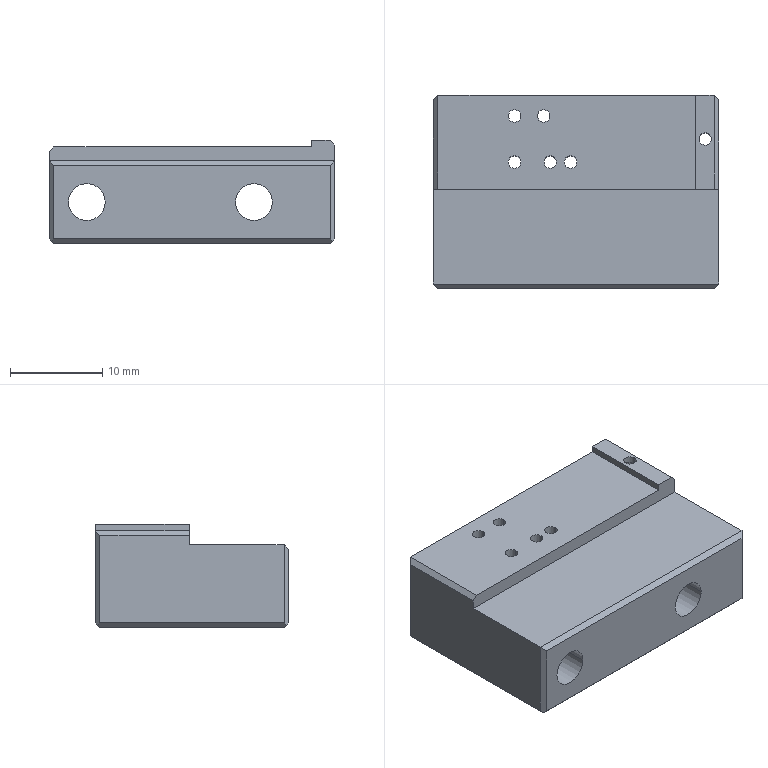Part | 1 solid | 45 faces | box 31 x 21 x 11.2 mm | volume 5581 mm3 | plane 23 | cylinder 22 | commonest cylinder face diameters 1.35 x14 4 x4 6 x2 6.5 x2
STEP:
#1=CARTESIAN_POINT('',(2008.3,163.,-157.1));
#2=VERTEX_POINT('',#1);
#3=CARTESIAN_POINT('',(2008.3,163.,-167.3));
#4=VERTEX_POINT('',#3);
#5=CARTESIAN_POINT('',(2008.3,163.,-162.2));
#6=DIRECTION('',(0.,0.,-1.));
#7=VECTOR('',#6,1000.);
#8=LINE('',#5,#7);
#9=EDGE_CURVE('',#2,#4,#8,.T.);
#10=ORIENTED_EDGE('',*,*,#9,.F.);
#11=CARTESIAN_POINT('',(2008.3,153.3,-157.1));
#12=VERTEX_POINT('',#11);
#13=CARTESIAN_POINT('',(2008.3,158.4,-157.1));
#14=DIRECTION('',(0.,1.,0.));
#15=VECTOR('',#14,1000.);
#16=LINE('',#13,#15);
#17=EDGE_CURVE('',#12,#2,#16,.T.);
#18=ORIENTED_EDGE('',*,*,#17,.F.);
#19=CARTESIAN_POINT('',(2008.3,153.3,-158.8));
#20=VERTEX_POINT('',#19);
#21=CARTESIAN_POINT('',(2008.3,153.3,-197.47));
#22=DIRECTION('',(0.,0.,-1.));
#23=VECTOR('',#22,1000.);
#24=LINE('',#21,#23);
#25=EDGE_CURVE('',#12,#20,#24,.T.);
#26=ORIENTED_EDGE('',*,*,#25,.T.);
#27=CARTESIAN_POINT('',(2008.3,143.,-158.8));
#28=VERTEX_POINT('',#27);
#29=CARTESIAN_POINT('',(2008.3,142.5,-158.8));
#30=DIRECTION('',(0.,-1.,0.));
#31=VECTOR('',#30,1000.);
#32=LINE('',#29,#31);
#33=EDGE_CURVE('',#20,#28,#32,.T.);
#34=ORIENTED_EDGE('',*,*,#33,.T.);
#35=CARTESIAN_POINT('',(2008.3,143.,-167.3));
#36=VERTEX_POINT('',#35);
#37=CARTESIAN_POINT('',(2008.3,143.,-163.05));
#38=DIRECTION('',(0.,0.,-1.));
#39=VECTOR('',#38,1000.);
#40=LINE('',#37,#39);
#41=EDGE_CURVE('',#28,#36,#40,.T.);
#42=ORIENTED_EDGE('',*,*,#41,.T.);
#43=CARTESIAN_POINT('',(2008.3,153.,-167.3));
#44=DIRECTION('',(0.,-1.,0.));
#45=VECTOR('',#44,1000.);
#46=LINE('',#43,#45);
#47=EDGE_CURVE('',#4,#36,#46,.T.);
#48=ORIENTED_EDGE('',*,*,#47,.F.);
#49=EDGE_LOOP('',(#10,#18,#26,#34,#42,#48));
#50=FACE_BOUND('',#49,.T.);
#51=CARTESIAN_POINT('',(2008.3,142.5,-213.5));
#52=DIRECTION('',(1.,0.,0.));
#53=DIRECTION('',(0.,1.,0.));
#54=AXIS2_PLACEMENT_3D('',#51,#52,#53);
#55=PLANE('',#54);
#56=ADVANCED_FACE('',(#50),#55,.T.);
#57=CARTESIAN_POINT('',(1977.8,143.,-167.8));
#58=VERTEX_POINT('',#57);
#59=CARTESIAN_POINT('',(1977.8,163.,-167.8));
#60=VERTEX_POINT('',#59);
#61=CARTESIAN_POINT('',(1977.8,153.,-167.8));
#62=DIRECTION('',(0.,1.,0.));
#63=VECTOR('',#62,1000.);
#64=LINE('',#61,#63);
#65=EDGE_CURVE('',#58,#60,#64,.T.);
#66=ORIENTED_EDGE('',*,*,#65,.T.);
#67=CARTESIAN_POINT('',(2007.8,163.,-167.8));
#68=VERTEX_POINT('',#67);
#69=CARTESIAN_POINT('',(1992.8,163.,-167.8));
#70=DIRECTION('',(1.,0.,0.));
#71=VECTOR('',#70,1000.);
#72=LINE('',#69,#71);
#73=EDGE_CURVE('',#60,#68,#72,.T.);
#74=ORIENTED_EDGE('',*,*,#73,.T.);
#75=CARTESIAN_POINT('',(2007.8,143.,-167.8));
#76=VERTEX_POINT('',#75);
#77=CARTESIAN_POINT('',(2007.8,153.,-167.8));
#78=DIRECTION('',(0.,-1.,0.));
#79=VECTOR('',#78,1000.);
#80=LINE('',#77,#79);
#81=EDGE_CURVE('',#68,#76,#80,.T.);
#82=ORIENTED_EDGE('',*,*,#81,.T.);
#83=CARTESIAN_POINT('',(1992.8,143.,-167.8));
#84=DIRECTION('',(-1.,0.,0.));
#85=VECTOR('',#84,1000.);
#86=LINE('',#83,#85);
#87=EDGE_CURVE('',#76,#58,#86,.T.);
#88=ORIENTED_EDGE('',*,*,#87,.T.);
#89=EDGE_LOOP('',(#66,#74,#82,#88));
#90=FACE_BOUND('',#89,.T.);
#91=CARTESIAN_POINT('',(1986.795,156.238,-167.8));
#92=VERTEX_POINT('',#91);
#93=CARTESIAN_POINT('',(1985.445,156.238,-167.8));
#94=VERTEX_POINT('',#93);
#95=CARTESIAN_POINT('',(1986.12,156.238,-167.8));
#96=DIRECTION('',(0.,0.,1.));
#97=DIRECTION('',(-1.,0.,0.));
#98=AXIS2_PLACEMENT_3D('',#95,#96,#97);
#99=CIRCLE('',#98,0.675);
#100=EDGE_CURVE('',#92,#94,#99,.T.);
#101=ORIENTED_EDGE('',*,*,#100,.T.);
#102=CARTESIAN_POINT('',(1986.12,156.238,-167.8));
#103=DIRECTION('',(0.,0.,1.));
#104=DIRECTION('',(-1.,0.,0.));
#105=AXIS2_PLACEMENT_3D('',#102,#103,#104);
#106=CIRCLE('',#105,0.675);
#107=EDGE_CURVE('',#94,#92,#106,.T.);
#108=ORIENTED_EDGE('',*,*,#107,.T.);
#109=EDGE_LOOP('',(#101,#108));
#110=FACE_BOUND('',#109,.T.);
#111=CARTESIAN_POINT('',(1992.885,156.238,-167.8));
#112=VERTEX_POINT('',#111);
#113=CARTESIAN_POINT('',(1991.535,156.238,-167.8));
#114=VERTEX_POINT('',#113);
#115=CARTESIAN_POINT('',(1992.21,156.238,-167.8));
#116=DIRECTION('',(0.,0.,1.));
#117=DIRECTION('',(-1.,0.,0.));
#118=AXIS2_PLACEMENT_3D('',#115,#116,#117);
#119=CIRCLE('',#118,0.675);
#120=EDGE_CURVE('',#112,#114,#119,.T.);
#121=ORIENTED_EDGE('',*,*,#120,.T.);
#122=CARTESIAN_POINT('',(1992.21,156.238,-167.8));
#123=DIRECTION('',(0.,0.,1.));
#124=DIRECTION('',(-1.,0.,0.));
#125=AXIS2_PLACEMENT_3D('',#122,#123,#124);
#126=CIRCLE('',#125,0.675);
#127=EDGE_CURVE('',#114,#112,#126,.T.);
#128=ORIENTED_EDGE('',*,*,#127,.T.);
#129=EDGE_LOOP('',(#121,#128));
#130=FACE_BOUND('',#129,.T.);
#131=CARTESIAN_POINT('',(2007.525,158.748,-167.8));
#132=VERTEX_POINT('',#131);
#133=CARTESIAN_POINT('',(2006.175,158.748,-167.8));
#134=VERTEX_POINT('',#133);
#135=CARTESIAN_POINT('',(2006.85,158.748,-167.8));
#136=DIRECTION('',(0.,0.,-1.));
#137=DIRECTION('',(-1.,0.,0.));
#138=AXIS2_PLACEMENT_3D('',#135,#136,#137);
#139=CIRCLE('',#138,0.675);
#140=EDGE_CURVE('',#132,#134,#139,.T.);
#141=ORIENTED_EDGE('',*,*,#140,.F.);
#142=CARTESIAN_POINT('',(2006.85,158.748,-167.8));
#143=DIRECTION('',(0.,0.,-1.));
#144=DIRECTION('',(-1.,0.,0.));
#145=AXIS2_PLACEMENT_3D('',#142,#143,#144);
#146=CIRCLE('',#145,0.675);
#147=EDGE_CURVE('',#134,#132,#146,.T.);
#148=ORIENTED_EDGE('',*,*,#147,.F.);
#149=EDGE_LOOP('',(#141,#148));
#150=FACE_BOUND('',#149,.T.);
#151=CARTESIAN_POINT('',(1986.795,161.259,-167.8));
#152=VERTEX_POINT('',#151);
#153=CARTESIAN_POINT('',(1985.445,161.259,-167.8));
#154=VERTEX_POINT('',#153);
#155=CARTESIAN_POINT('',(1986.12,161.259,-167.8));
#156=DIRECTION('',(0.,0.,1.));
#157=DIRECTION('',(-1.,0.,0.));
#158=AXIS2_PLACEMENT_3D('',#155,#156,#157);
#159=CIRCLE('',#158,0.675);
#160=EDGE_CURVE('',#152,#154,#159,.T.);
#161=ORIENTED_EDGE('',*,*,#160,.T.);
#162=CARTESIAN_POINT('',(1986.12,161.259,-167.8));
#163=DIRECTION('',(0.,0.,1.));
#164=DIRECTION('',(-1.,0.,0.));
#165=AXIS2_PLACEMENT_3D('',#162,#163,#164);
#166=CIRCLE('',#165,0.675);
#167=EDGE_CURVE('',#154,#152,#166,.T.);
#168=ORIENTED_EDGE('',*,*,#167,.T.);
#169=EDGE_LOOP('',(#161,#168));
#170=FACE_BOUND('',#169,.T.);
#171=CARTESIAN_POINT('',(1989.958,161.259,-167.8));
#172=VERTEX_POINT('',#171);
#173=CARTESIAN_POINT('',(1988.608,161.259,-167.8));
#174=VERTEX_POINT('',#173);
#175=CARTESIAN_POINT('',(1989.283,161.259,-167.8));
#176=DIRECTION('',(0.,0.,1.));
#177=DIRECTION('',(-1.,0.,0.));
#178=AXIS2_PLACEMENT_3D('',#175,#176,#177);
#179=CIRCLE('',#178,0.675);
#180=EDGE_CURVE('',#172,#174,#179,.T.);
#181=ORIENTED_EDGE('',*,*,#180,.T.);
#182=CARTESIAN_POINT('',(1989.283,161.259,-167.8));
#183=DIRECTION('',(0.,0.,1.));
#184=DIRECTION('',(-1.,0.,0.));
#185=AXIS2_PLACEMENT_3D('',#182,#183,#184);
#186=CIRCLE('',#185,0.675);
#187=EDGE_CURVE('',#174,#172,#186,.T.);
#188=ORIENTED_EDGE('',*,*,#187,.T.);
#189=EDGE_LOOP('',(#181,#188));
#190=FACE_BOUND('',#189,.T.);
#191=CARTESIAN_POINT('',(1990.685,156.238,-167.8));
#192=VERTEX_POINT('',#191);
#193=CARTESIAN_POINT('',(1989.335,156.238,-167.8));
#194=VERTEX_POINT('',#193);
#195=CARTESIAN_POINT('',(1990.01,156.238,-167.8));
#196=DIRECTION('',(0.,0.,1.));
#197=DIRECTION('',(-1.,0.,0.));
#198=AXIS2_PLACEMENT_3D('',#195,#196,#197);
#199=CIRCLE('',#198,0.675);
#200=EDGE_CURVE('',#192,#194,#199,.T.);
#201=ORIENTED_EDGE('',*,*,#200,.T.);
#202=CARTESIAN_POINT('',(1990.01,156.238,-167.8));
#203=DIRECTION('',(0.,0.,1.));
#204=DIRECTION('',(-1.,0.,0.));
#205=AXIS2_PLACEMENT_3D('',#202,#203,#204);
#206=CIRCLE('',#205,0.675);
#207=EDGE_CURVE('',#194,#192,#206,.T.);
#208=ORIENTED_EDGE('',*,*,#207,.T.);
#209=EDGE_LOOP('',(#201,#208));
#210=FACE_BOUND('',#209,.T.);
#211=CARTESIAN_POINT('',(2010.,142.5,-167.8));
#212=DIRECTION('',(0.,0.,-1.));
#213=DIRECTION('',(0.,-1.,0.));
#214=AXIS2_PLACEMENT_3D('',#211,#212,#213);
#215=PLANE('',#214);
#216=ADVANCED_FACE('',(#90,#110,#130,#150,#170,#190,#210),#215,.T.);
#217=CARTESIAN_POINT('',(1977.3,163.,-157.8));
#218=VERTEX_POINT('',#217);
#219=CARTESIAN_POINT('',(1977.3,153.3,-157.8));
#220=VERTEX_POINT('',#219);
#221=CARTESIAN_POINT('',(1977.3,158.4,-157.8));
#222=DIRECTION('',(0.,-1.,0.));
#223=VECTOR('',#222,1000.);
#224=LINE('',#221,#223);
#225=EDGE_CURVE('',#218,#220,#224,.T.);
#226=ORIENTED_EDGE('',*,*,#225,.F.);
#227=CARTESIAN_POINT('',(1977.3,163.,-167.3));
#228=VERTEX_POINT('',#227);
#229=CARTESIAN_POINT('',(1977.3,163.,-162.55));
#230=DIRECTION('',(0.,0.,1.));
#231=VECTOR('',#230,1000.);
#232=LINE('',#229,#231);
#233=EDGE_CURVE('',#228,#218,#232,.T.);
#234=ORIENTED_EDGE('',*,*,#233,.F.);
#235=CARTESIAN_POINT('',(1977.3,143.,-167.3));
#236=VERTEX_POINT('',#235);
#237=CARTESIAN_POINT('',(1977.3,153.,-167.3));
#238=DIRECTION('',(0.,1.,0.));
#239=VECTOR('',#238,1000.);
#240=LINE('',#237,#239);
#241=EDGE_CURVE('',#236,#228,#240,.T.);
#242=ORIENTED_EDGE('',*,*,#241,.F.);
#243=CARTESIAN_POINT('',(1977.3,143.,-158.8));
#244=VERTEX_POINT('',#243);
#245=CARTESIAN_POINT('',(1977.3,143.,-163.05));
#246=DIRECTION('',(0.,0.,1.));
#247=VECTOR('',#246,1000.);
#248=LINE('',#245,#247);
#249=EDGE_CURVE('',#236,#244,#248,.T.);
#250=ORIENTED_EDGE('',*,*,#249,.T.);
#251=CARTESIAN_POINT('',(1977.3,153.3,-158.8));
#252=VERTEX_POINT('',#251);
#253=CARTESIAN_POINT('',(1977.3,142.5,-158.8));
#254=DIRECTION('',(0.,1.,0.));
#255=VECTOR('',#254,1000.);
#256=LINE('',#253,#255);
#257=EDGE_CURVE('',#244,#252,#256,.T.);
#258=ORIENTED_EDGE('',*,*,#257,.T.);
#259=CARTESIAN_POINT('',(1977.3,153.3,-197.47));
#260=DIRECTION('',(0.,0.,1.));
#261=VECTOR('',#260,1000.);
#262=LINE('',#259,#261);
#263=EDGE_CURVE('',#252,#220,#262,.T.);
#264=ORIENTED_EDGE('',*,*,#263,.T.);
#265=EDGE_LOOP('',(#226,#234,#242,#250,#258,#264));
#266=FACE_BOUND('',#265,.T.);
#267=CARTESIAN_POINT('',(1977.3,142.5,-205.7));
#268=DIRECTION('',(-1.,0.,0.));
#269=DIRECTION('',(0.,0.,1.));
#270=AXIS2_PLACEMENT_3D('',#267,#268,#269);
#271=PLANE('',#270);
#272=ADVANCED_FACE('',(#266),#271,.T.);
#273=CARTESIAN_POINT('',(2005.8,153.3,-156.6));
#274=VERTEX_POINT('',#273);
#275=CARTESIAN_POINT('',(2005.8,153.3,-157.3));
#276=VERTEX_POINT('',#275);
#277=CARTESIAN_POINT('',(2005.8,153.3,-197.47));
#278=DIRECTION('',(0.,0.,-1.));
#279=VECTOR('',#278,1000.);
#280=LINE('',#277,#279);
#281=EDGE_CURVE('',#274,#276,#280,.T.);
#282=ORIENTED_EDGE('',*,*,#281,.F.);
#283=CARTESIAN_POINT('',(2005.8,163.5,-156.6));
#284=VERTEX_POINT('',#283);
#285=CARTESIAN_POINT('',(2005.8,142.5,-156.6));
#286=DIRECTION('',(0.,1.,0.));
#287=VECTOR('',#286,1000.);
#288=LINE('',#285,#287);
#289=EDGE_CURVE('',#274,#284,#288,.T.);
#290=ORIENTED_EDGE('',*,*,#289,.T.);
#291=CARTESIAN_POINT('',(2005.8,163.5,-157.3));
#292=VERTEX_POINT('',#291);
#293=CARTESIAN_POINT('',(2005.8,163.5,-197.47));
#294=DIRECTION('',(0.,0.,-1.));
#295=VECTOR('',#294,1000.);
#296=LINE('',#293,#295);
#297=EDGE_CURVE('',#284,#292,#296,.T.);
#298=ORIENTED_EDGE('',*,*,#297,.T.);
#299=CARTESIAN_POINT('',(2005.8,142.5,-157.3));
#300=DIRECTION('',(0.,-1.,0.));
#301=VECTOR('',#300,1000.);
#302=LINE('',#299,#301);
#303=EDGE_CURVE('',#292,#276,#302,.T.);
#304=ORIENTED_EDGE('',*,*,#303,.T.);
#305=EDGE_LOOP('',(#282,#290,#298,#304));
#306=FACE_BOUND('',#305,.T.);
#307=CARTESIAN_POINT('',(2005.8,142.5,-157.3));
#308=DIRECTION('',(-1.,0.,0.));
#309=DIRECTION('',(0.,0.,1.));
#310=AXIS2_PLACEMENT_3D('',#307,#308,#309);
#311=PLANE('',#310);
#312=ADVANCED_FACE('',(#306),#311,.T.);
#313=CARTESIAN_POINT('',(1986.795,161.259,-157.3));
#314=VERTEX_POINT('',#313);
#315=CARTESIAN_POINT('',(1985.445,161.259,-157.3));
#316=VERTEX_POINT('',#315);
#317=CARTESIAN_POINT('',(1986.12,161.259,-157.3));
#318=DIRECTION('',(0.,0.,1.));
#319=DIRECTION('',(-1.,0.,0.));
#320=AXIS2_PLACEMENT_3D('',#317,#318,#319);
#321=CIRCLE('',#320,0.675);
#322=EDGE_CURVE('',#314,#316,#321,.T.);
#323=ORIENTED_EDGE('',*,*,#322,.T.);
#324=CARTESIAN_POINT('',(1985.445,161.259,-157.3));
#325=DIRECTION('',(0.,0.,1.));
#326=VECTOR('',#325,1000.);
#327=LINE('',#324,#326);
#328=EDGE_CURVE('',#316,#154,#327,.F.);
#329=ORIENTED_EDGE('',*,*,#328,.T.);
#330=ORIENTED_EDGE('',*,*,#160,.F.);
#331=CARTESIAN_POINT('',(1986.795,161.259,-157.3));
#332=DIRECTION('',(0.,0.,1.));
#333=VECTOR('',#332,1000.);
#334=LINE('',#331,#333);
#335=EDGE_CURVE('',#314,#152,#334,.F.);
#336=ORIENTED_EDGE('',*,*,#335,.F.);
#337=EDGE_LOOP('',(#323,#329,#330,#336));
#338=FACE_BOUND('',#337,.T.);
#339=CARTESIAN_POINT('',(1986.12,161.259,-157.3));
#340=DIRECTION('',(0.,0.,1.));
#341=DIRECTION('',(-1.,0.,0.));
#342=AXIS2_PLACEMENT_3D('',#339,#340,#341);
#343=CYLINDRICAL_SURFACE('',#342,0.675);
#344=ADVANCED_FACE('',(#338),#343,.F.);
#345=CARTESIAN_POINT('',(1989.958,161.259,-157.3));
#346=VERTEX_POINT('',#345);
#347=CARTESIAN_POINT('',(1988.608,161.259,-157.3));
#348=VERTEX_POINT('',#347);
#349=CARTESIAN_POINT('',(1989.283,161.259,-157.3));
#350=DIRECTION('',(0.,0.,1.));
#351=DIRECTION('',(-1.,0.,0.));
#352=AXIS2_PLACEMENT_3D('',#349,#350,#351);
#353=CIRCLE('',#352,0.675);
#354=EDGE_CURVE('',#346,#348,#353,.T.);
#355=ORIENTED_EDGE('',*,*,#354,.T.);
#356=CARTESIAN_POINT('',(1988.608,161.259,-157.3));
#357=DIRECTION('',(0.,0.,1.));
#358=VECTOR('',#357,1000.);
#359=LINE('',#356,#358);
#360=EDGE_CURVE('',#348,#174,#359,.F.);
#361=ORIENTED_EDGE('',*,*,#360,.T.);
#362=ORIENTED_EDGE('',*,*,#180,.F.);
#363=CARTESIAN_POINT('',(1989.958,161.259,-157.3));
#364=DIRECTION('',(0.,0.,1.));
#365=VECTOR('',#364,1000.);
#366=LINE('',#363,#365);
#367=EDGE_CURVE('',#346,#172,#366,.F.);
#368=ORIENTED_EDGE('',*,*,#367,.F.);
#369=EDGE_LOOP('',(#355,#361,#362,#368));
#370=FACE_BOUND('',#369,.T.);
#371=CARTESIAN_POINT('',(1989.283,161.259,-157.3));
#372=DIRECTION('',(0.,0.,1.));
#373=DIRECTION('',(-1.,0.,0.));
#374=AXIS2_PLACEMENT_3D('',#371,#372,#373);
#375=CYLINDRICAL_SURFACE('',#374,0.675);
#376=ADVANCED_FACE('',(#370),#375,.F.);
#377=CARTESIAN_POINT('',(1990.685,156.238,-157.3));
#378=VERTEX_POINT('',#377);
#379=CARTESIAN_POINT('',(1989.335,156.238,-157.3));
#380=VERTEX_POINT('',#379);
#381=CARTESIAN_POINT('',(1990.01,156.238,-157.3));
#382=DIRECTION('',(0.,0.,1.));
#383=DIRECTION('',(-1.,0.,0.));
#384=AXIS2_PLACEMENT_3D('',#381,#382,#383);
#385=CIRCLE('',#384,0.675);
#386=EDGE_CURVE('',#378,#380,#385,.T.);
#387=ORIENTED_EDGE('',*,*,#386,.T.);
#388=CARTESIAN_POINT('',(1989.335,156.238,-157.3));
#389=DIRECTION('',(0.,0.,1.));
#390=VECTOR('',#389,1000.);
#391=LINE('',#388,#390);
#392=EDGE_CURVE('',#380,#194,#391,.F.);
#393=ORIENTED_EDGE('',*,*,#392,.T.);
#394=ORIENTED_EDGE('',*,*,#200,.F.);
#395=CARTESIAN_POINT('',(1990.685,156.238,-157.3));
#396=DIRECTION('',(0.,0.,1.));
#397=VECTOR('',#396,1000.);
#398=LINE('',#395,#397);
#399=EDGE_CURVE('',#378,#192,#398,.F.);
#400=ORIENTED_EDGE('',*,*,#399,.F.);
#401=EDGE_LOOP('',(#387,#393,#394,#400));
#402=FACE_BOUND('',#401,.T.);
#403=CARTESIAN_POINT('',(1990.01,156.238,-157.3));
#404=DIRECTION('',(0.,0.,1.));
#405=DIRECTION('',(-1.,0.,0.));
#406=AXIS2_PLACEMENT_3D('',#403,#404,#405);
#407=CYLINDRICAL_SURFACE('',#406,0.675);
#408=ADVANCED_FACE('',(#402),#407,.F.);
#409=CARTESIAN_POINT('',(1986.795,156.238,-157.3));
#410=VERTEX_POINT('',#409);
#411=CARTESIAN_POINT('',(1985.445,156.238,-157.3));
#412=VERTEX_POINT('',#411);
#413=CARTESIAN_POINT('',(1986.12,156.238,-157.3));
#414=DIRECTION('',(0.,0.,1.));
#415=DIRECTION('',(-1.,0.,0.));
#416=AXIS2_PLACEMENT_3D('',#413,#414,#415);
#417=CIRCLE('',#416,0.675);
#418=EDGE_CURVE('',#410,#412,#417,.T.);
#419=ORIENTED_EDGE('',*,*,#418,.T.);
#420=CARTESIAN_POINT('',(1985.445,156.238,-157.3));
#421=DIRECTION('',(0.,0.,1.));
#422=VECTOR('',#421,1000.);
#423=LINE('',#420,#422);
#424=EDGE_CURVE('',#412,#94,#423,.F.);
#425=ORIENTED_EDGE('',*,*,#424,.T.);
#426=ORIENTED_EDGE('',*,*,#100,.F.);
#427=CARTESIAN_POINT('',(1986.795,156.238,-157.3));
#428=DIRECTION('',(0.,0.,1.));
#429=VECTOR('',#428,1000.);
#430=LINE('',#427,#429);
#431=EDGE_CURVE('',#410,#92,#430,.F.);
#432=ORIENTED_EDGE('',*,*,#431,.F.);
#433=EDGE_LOOP('',(#419,#425,#426,#432));
#434=FACE_BOUND('',#433,.T.);
#435=CARTESIAN_POINT('',(1986.12,156.238,-157.3));
#436=DIRECTION('',(0.,0.,1.));
#437=DIRECTION('',(-1.,0.,0.));
#438=AXIS2_PLACEMENT_3D('',#435,#436,#437);
#439=CYLINDRICAL_SURFACE('',#438,0.675);
#440=ADVANCED_FACE('',(#434),#439,.F.);
#441=CARTESIAN_POINT('',(1992.885,156.238,-157.3));
#442=VERTEX_POINT('',#441);
#443=CARTESIAN_POINT('',(1991.535,156.238,-157.3));
#444=VERTEX_POINT('',#443);
#445=CARTESIAN_POINT('',(1992.21,156.238,-157.3));
#446=DIRECTION('',(0.,0.,1.));
#447=DIRECTION('',(-1.,0.,0.));
#448=AXIS2_PLACEMENT_3D('',#445,#446,#447);
#449=CIRCLE('',#448,0.675);
#450=EDGE_CURVE('',#442,#444,#449,.T.);
#451=ORIENTED_EDGE('',*,*,#450,.T.);
#452=CARTESIAN_POINT('',(1991.535,156.238,-157.3));
#453=DIRECTION('',(0.,0.,1.));
#454=VECTOR('',#453,1000.);
#455=LINE('',#452,#454);
#456=EDGE_CURVE('',#444,#114,#455,.F.);
#457=ORIENTED_EDGE('',*,*,#456,.T.);
#458=ORIENTED_EDGE('',*,*,#120,.F.);
#459=CARTESIAN_POINT('',(1992.885,156.238,-157.3));
#460=DIRECTION('',(0.,0.,1.));
#461=VECTOR('',#460,1000.);
#462=LINE('',#459,#461);
#463=EDGE_CURVE('',#442,#112,#462,.F.);
#464=ORIENTED_EDGE('',*,*,#463,.F.);
#465=EDGE_LOOP('',(#451,#457,#458,#464));
#466=FACE_BOUND('',#465,.T.);
#467=CARTESIAN_POINT('',(1992.21,156.238,-157.3));
#468=DIRECTION('',(0.,0.,1.));
#469=DIRECTION('',(-1.,0.,0.));
#470=AXIS2_PLACEMENT_3D('',#467,#468,#469);
#471=CYLINDRICAL_SURFACE('',#470,0.675);
#472=ADVANCED_FACE('',(#466),#471,.F.);
#473=CARTESIAN_POINT('',(2007.525,158.748,-157.3));
#474=VERTEX_POINT('',#473);
#475=CARTESIAN_POINT('',(2006.175,158.748,-157.3));
#476=VERTEX_POINT('',#475);
#477=CARTESIAN_POINT('',(2006.85,158.748,-157.3));
#478=DIRECTION('',(0.,0.,-1.));
#479=DIRECTION('',(-1.,0.,0.));
#480=AXIS2_PLACEMENT_3D('',#477,#478,#479);
#481=CIRCLE('',#480,0.675);
#482=EDGE_CURVE('',#474,#476,#481,.T.);
#483=ORIENTED_EDGE('',*,*,#482,.F.);
#484=CARTESIAN_POINT('',(2007.525,158.748,-157.3));
#485=DIRECTION('',(0.,0.,1.));
#486=VECTOR('',#485,1000.);
#487=LINE('',#484,#486);
#488=EDGE_CURVE('',#474,#132,#487,.F.);
#489=ORIENTED_EDGE('',*,*,#488,.T.);
#490=ORIENTED_EDGE('',*,*,#140,.T.);
#491=CARTESIAN_POINT('',(2006.175,158.748,-157.3));
#492=DIRECTION('',(0.,0.,1.));
#493=VECTOR('',#492,1000.);
#494=LINE('',#491,#493);
#495=EDGE_CURVE('',#476,#134,#494,.F.);
#496=ORIENTED_EDGE('',*,*,#495,.F.);
#497=EDGE_LOOP('',(#483,#489,#490,#496));
#498=FACE_BOUND('',#497,.T.);
#499=CARTESIAN_POINT('',(2006.85,158.748,-157.3));
#500=DIRECTION('',(0.,0.,1.));
#501=DIRECTION('',(-1.,0.,0.));
#502=AXIS2_PLACEMENT_3D('',#499,#500,#501);
#503=CYLINDRICAL_SURFACE('',#502,0.675);
#504=ADVANCED_FACE('',(#498),#503,.F.);
#505=CARTESIAN_POINT('',(1977.8,153.3,-157.3));
#506=VERTEX_POINT('',#505);
#507=CARTESIAN_POINT('',(1983.678,153.3,-157.3));
#508=DIRECTION('',(-1.,0.,0.));
#509=VECTOR('',#508,1000.);
#510=LINE('',#507,#509);
#511=EDGE_CURVE('',#276,#506,#510,.T.);
#512=ORIENTED_EDGE('',*,*,#511,.F.);
#513=ORIENTED_EDGE('',*,*,#303,.F.);
#514=CARTESIAN_POINT('',(1977.8,163.5,-157.3));
#515=VERTEX_POINT('',#514);
#516=CARTESIAN_POINT('',(1983.678,163.5,-157.3));
#517=DIRECTION('',(-1.,0.,0.));
#518=VECTOR('',#517,1000.);
#519=LINE('',#516,#518);
#520=EDGE_CURVE('',#292,#515,#519,.T.);
#521=ORIENTED_EDGE('',*,*,#520,.T.);
#522=CARTESIAN_POINT('',(1977.8,158.4,-157.3));
#523=DIRECTION('',(0.,-1.,0.));
#524=VECTOR('',#523,1000.);
#525=LINE('',#522,#524);
#526=EDGE_CURVE('',#515,#506,#525,.T.);
#527=ORIENTED_EDGE('',*,*,#526,.T.);
#528=EDGE_LOOP('',(#512,#513,#521,#527));
#529=FACE_BOUND('',#528,.T.);
#530=ORIENTED_EDGE('',*,*,#450,.F.);
#531=CARTESIAN_POINT('',(1992.21,156.238,-157.3));
#532=DIRECTION('',(0.,0.,1.));
#533=DIRECTION('',(-1.,0.,0.));
#534=AXIS2_PLACEMENT_3D('',#531,#532,#533);
#535=CIRCLE('',#534,0.675);
#536=EDGE_CURVE('',#444,#442,#535,.T.);
#537=ORIENTED_EDGE('',*,*,#536,.F.);
#538=EDGE_LOOP('',(#530,#537));
#539=FACE_BOUND('',#538,.T.);
#540=ORIENTED_EDGE('',*,*,#322,.F.);
#541=CARTESIAN_POINT('',(1986.12,161.259,-157.3));
#542=DIRECTION('',(0.,0.,1.));
#543=DIRECTION('',(-1.,0.,0.));
#544=AXIS2_PLACEMENT_3D('',#541,#542,#543);
#545=CIRCLE('',#544,0.675);
#546=EDGE_CURVE('',#316,#314,#545,.T.);
#547=ORIENTED_EDGE('',*,*,#546,.F.);
#548=EDGE_LOOP('',(#540,#547));
#549=FACE_BOUND('',#548,.T.);
#550=ORIENTED_EDGE('',*,*,#354,.F.);
#551=CARTESIAN_POINT('',(1989.283,161.259,-157.3));
#552=DIRECTION('',(0.,0.,1.));
#553=DIRECTION('',(-1.,0.,0.));
#554=AXIS2_PLACEMENT_3D('',#551,#552,#553);
#555=CIRCLE('',#554,0.675);
#556=EDGE_CURVE('',#348,#346,#555,.T.);
#557=ORIENTED_EDGE('',*,*,#556,.F.);
#558=EDGE_LOOP('',(#550,#557));
#559=FACE_BOUND('',#558,.T.);
#560=ORIENTED_EDGE('',*,*,#386,.F.);
#561=CARTESIAN_POINT('',(1990.01,156.238,-157.3));
#562=DIRECTION('',(0.,0.,1.));
#563=DIRECTION('',(-1.,0.,0.));
#564=AXIS2_PLACEMENT_3D('',#561,#562,#563);
#565=CIRCLE('',#564,0.675);
#566=EDGE_CURVE('',#380,#378,#565,.T.);
#567=ORIENTED_EDGE('',*,*,#566,.F.);
#568=EDGE_LOOP('',(#560,#567));
#569=FACE_BOUND('',#568,.T.);
#570=ORIENTED_EDGE('',*,*,#418,.F.);
#571=CARTESIAN_POINT('',(1986.12,156.238,-157.3));
#572=DIRECTION('',(0.,0.,1.));
#573=DIRECTION('',(-1.,0.,0.));
#574=AXIS2_PLACEMENT_3D('',#571,#572,#573);
#575=CIRCLE('',#574,0.675);
#576=EDGE_CURVE('',#412,#410,#575,.T.);
#577=ORIENTED_EDGE('',*,*,#576,.F.);
#578=EDGE_LOOP('',(#570,#577));
#579=FACE_BOUND('',#578,.T.);
#580=CARTESIAN_POINT('',(2010.3,142.5,-157.3));
#581=DIRECTION('',(0.,0.,1.));
#582=DIRECTION('',(1.,0.,0.));
#583=AXIS2_PLACEMENT_3D('',#580,#581,#582);
#584=PLANE('',#583);
#585=ADVANCED_FACE('',(#529,#539,#549,#559,#569,#579),#584,.T.);
#586=CARTESIAN_POINT('',(2007.8,153.3,-156.6));
#587=VERTEX_POINT('',#586);
#588=CARTESIAN_POINT('',(2007.8,163.5,-156.6));
#589=VERTEX_POINT('',#588);
#590=CARTESIAN_POINT('',(2007.8,158.4,-156.6));
#591=DIRECTION('',(0.,1.,0.));
#592=VECTOR('',#591,1000.);
#593=LINE('',#590,#592);
#594=EDGE_CURVE('',#587,#589,#593,.T.);
#595=ORIENTED_EDGE('',*,*,#594,.T.);
#596=CARTESIAN_POINT('',(1983.678,163.5,-156.6));
#597=DIRECTION('',(-1.,0.,0.));
#598=VECTOR('',#597,1000.);
#599=LINE('',#596,#598);
#600=EDGE_CURVE('',#589,#284,#599,.T.);
#601=ORIENTED_EDGE('',*,*,#600,.T.);
#602=ORIENTED_EDGE('',*,*,#289,.F.);
#603=CARTESIAN_POINT('',(1983.678,153.3,-156.6));
#604=DIRECTION('',(-1.,0.,0.));
#605=VECTOR('',#604,1000.);
#606=LINE('',#603,#605);
#607=EDGE_CURVE('',#587,#274,#606,.T.);
#608=ORIENTED_EDGE('',*,*,#607,.F.);
#609=EDGE_LOOP('',(#595,#601,#602,#608));
#610=FACE_BOUND('',#609,.T.);
#611=CARTESIAN_POINT('',(2007.525,158.748,-156.6));
#612=VERTEX_POINT('',#611);
#613=CARTESIAN_POINT('',(2006.175,158.748,-156.6));
#614=VERTEX_POINT('',#613);
#615=CARTESIAN_POINT('',(2006.85,158.748,-156.6));
#616=DIRECTION('',(0.,0.,-1.));
#617=DIRECTION('',(-1.,0.,0.));
#618=AXIS2_PLACEMENT_3D('',#615,#616,#617);
#619=CIRCLE('',#618,0.675);
#620=EDGE_CURVE('',#612,#614,#619,.T.);
#621=ORIENTED_EDGE('',*,*,#620,.T.);
#622=CARTESIAN_POINT('',(2006.85,158.748,-156.6));
#623=DIRECTION('',(0.,0.,-1.));
#624=DIRECTION('',(-1.,0.,0.));
#625=AXIS2_PLACEMENT_3D('',#622,#623,#624);
#626=CIRCLE('',#625,0.675);
#627=EDGE_CURVE('',#614,#612,#626,.T.);
#628=ORIENTED_EDGE('',*,*,#627,.T.);
#629=EDGE_LOOP('',(#621,#628));
#630=FACE_BOUND('',#629,.T.);
#631=CARTESIAN_POINT('',(2008.974,161.53,-156.6));
#632=DIRECTION('',(0.,0.,1.));
#633=DIRECTION('',(1.,0.,0.));
#634=AXIS2_PLACEMENT_3D('',#631,#632,#633);
#635=PLANE('',#634);
#636=ADVANCED_FACE('',(#610,#630),#635,.T.);
#637=ORIENTED_EDGE('',*,*,#594,.F.);
#638=CARTESIAN_POINT('',(2048.67,153.3,-197.47));
#639=DIRECTION('',(-0.7071,0.,0.7071));
#640=VECTOR('',#639,1000.);
#641=LINE('',#638,#640);
#642=EDGE_CURVE('',#12,#587,#641,.T.);
#643=ORIENTED_EDGE('',*,*,#642,.F.);
#644=ORIENTED_EDGE('',*,*,#17,.T.);
#645=CARTESIAN_POINT('',(2028.8,142.5,-177.6));
#646=DIRECTION('',(-0.5774,0.5774,0.5774));
#647=VECTOR('',#646,1000.);
#648=LINE('',#645,#647);
#649=EDGE_CURVE('',#2,#589,#648,.T.);
#650=ORIENTED_EDGE('',*,*,#649,.T.);
#651=EDGE_LOOP('',(#637,#643,#644,#650));
#652=FACE_BOUND('',#651,.T.);
#653=CARTESIAN_POINT('',(2008.05,158.4,-156.85));
#654=DIRECTION('',(0.7071,0.,0.7071));
#655=DIRECTION('',(0.,-1.,0.));
#656=AXIS2_PLACEMENT_3D('',#653,#654,#655);
#657=PLANE('',#656);
#658=ADVANCED_FACE('',(#652),#657,.T.);
#659=ORIENTED_EDGE('',*,*,#25,.F.);
#660=ORIENTED_EDGE('',*,*,#642,.T.);
#661=ORIENTED_EDGE('',*,*,#607,.T.);
#662=ORIENTED_EDGE('',*,*,#281,.T.);
#663=ORIENTED_EDGE('',*,*,#511,.T.);
#664=CARTESIAN_POINT('',(1937.63,153.3,-197.47));
#665=DIRECTION('',(0.7071,0.,0.7071));
#666=VECTOR('',#665,1000.);
#667=LINE('',#664,#666);
#668=EDGE_CURVE('',#220,#506,#667,.T.);
#669=ORIENTED_EDGE('',*,*,#668,.F.);
#670=ORIENTED_EDGE('',*,*,#263,.F.);
#671=CARTESIAN_POINT('',(1983.678,153.3,-158.8));
#672=DIRECTION('',(-1.,0.,0.));
#673=VECTOR('',#672,1000.);
#674=LINE('',#671,#673);
#675=EDGE_CURVE('',#20,#252,#674,.T.);
#676=ORIENTED_EDGE('',*,*,#675,.F.);
#677=EDGE_LOOP('',(#659,#660,#661,#662,#663,#669,#670,#676));
#678=FACE_BOUND('',#677,.T.);
#679=CARTESIAN_POINT('',(1975.1,153.3,-156.6));
#680=DIRECTION('',(0.,1.,0.));
#681=DIRECTION('',(1.,0.,0.));
#682=AXIS2_PLACEMENT_3D('',#679,#680,#681);
#683=PLANE('',#682);
#684=ADVANCED_FACE('',(#678),#683,.F.);
#685=ORIENTED_EDGE('',*,*,#257,.F.);
#686=CARTESIAN_POINT('',(1992.8,143.,-158.8));
#687=DIRECTION('',(-1.,0.,0.));
#688=VECTOR('',#687,1000.);
#689=LINE('',#686,#688);
#690=EDGE_CURVE('',#28,#244,#689,.T.);
#691=ORIENTED_EDGE('',*,*,#690,.F.);
#692=ORIENTED_EDGE('',*,*,#33,.F.);
#693=ORIENTED_EDGE('',*,*,#675,.T.);
#694=EDGE_LOOP('',(#685,#691,#692,#693));
#695=FACE_BOUND('',#694,.T.);
#696=CARTESIAN_POINT('',(1975.1,153.3,-158.8));
#697=DIRECTION('',(0.,0.,-1.));
#698=DIRECTION('',(0.,-1.,0.));
#699=AXIS2_PLACEMENT_3D('',#696,#697,#698);
#700=PLANE('',#699);
#701=ADVANCED_FACE('',(#695),#700,.F.);
#702=ORIENTED_EDGE('',*,*,#47,.T.);
#703=CARTESIAN_POINT('',(2008.05,142.75,-167.55));
#704=VERTEX_POINT('',#703);
#705=CARTESIAN_POINT('',(2007.8,142.5,-167.8));
#706=DIRECTION('',(0.5774,0.5774,0.5774));
#707=VECTOR('',#706,1000.);
#708=LINE('',#705,#707);
#709=EDGE_CURVE('',#704,#36,#708,.T.);
#710=ORIENTED_EDGE('',*,*,#709,.F.);
#711=CARTESIAN_POINT('',(1983.678,167.122,-191.922));
#712=DIRECTION('',(0.5774,-0.5774,0.5774));
#713=VECTOR('',#712,1000.);
#714=LINE('',#711,#713);
#715=EDGE_CURVE('',#76,#704,#714,.T.);
#716=ORIENTED_EDGE('',*,*,#715,.F.);
#717=ORIENTED_EDGE('',*,*,#81,.F.);
#718=CARTESIAN_POINT('',(2008.05,163.25,-167.55));
#719=VERTEX_POINT('',#718);
#720=CARTESIAN_POINT('',(1983.678,138.878,-191.922));
#721=DIRECTION('',(0.5774,0.5774,0.5774));
#722=VECTOR('',#721,1000.);
#723=LINE('',#720,#722);
#724=EDGE_CURVE('',#68,#719,#723,.T.);
#725=ORIENTED_EDGE('',*,*,#724,.T.);
#726=CARTESIAN_POINT('',(2028.8,142.5,-146.8));
#727=DIRECTION('',(0.5774,-0.5774,0.5774));
#728=VECTOR('',#727,1000.);
#729=LINE('',#726,#728);
#730=EDGE_CURVE('',#719,#4,#729,.T.);
#731=ORIENTED_EDGE('',*,*,#730,.T.);
#732=EDGE_LOOP('',(#702,#710,#716,#717,#725,#731));
#733=FACE_BOUND('',#732,.T.);
#734=CARTESIAN_POINT('',(2008.05,153.,-167.55));
#735=DIRECTION('',(-0.7071,0.,0.7071));
#736=DIRECTION('',(0.,1.,0.));
#737=AXIS2_PLACEMENT_3D('',#734,#735,#736);
#738=PLANE('',#737);
#739=ADVANCED_FACE('',(#733),#738,.F.);
#740=ORIENTED_EDGE('',*,*,#9,.T.);
#741=ORIENTED_EDGE('',*,*,#730,.F.);
#742=CARTESIAN_POINT('',(2007.8,163.5,-167.3));
#743=VERTEX_POINT('',#742);
#744=CARTESIAN_POINT('',(2028.8,142.5,-188.3));
#745=DIRECTION('',(-0.5774,0.5774,0.5774));
#746=VECTOR('',#745,1000.);
#747=LINE('',#744,#746);
#748=EDGE_CURVE('',#719,#743,#747,.T.);
#749=ORIENTED_EDGE('',*,*,#748,.T.);
#750=CARTESIAN_POINT('',(2007.8,163.5,-162.2));
#751=DIRECTION('',(0.,0.,-1.));
#752=VECTOR('',#751,1000.);
#753=LINE('',#750,#752);
#754=EDGE_CURVE('',#589,#743,#753,.T.);
#755=ORIENTED_EDGE('',*,*,#754,.F.);
#756=ORIENTED_EDGE('',*,*,#649,.F.);
#757=EDGE_LOOP('',(#740,#741,#749,#755,#756));
#758=FACE_BOUND('',#757,.T.);
#759=CARTESIAN_POINT('',(2008.05,163.25,-162.2));
#760=DIRECTION('',(-0.7071,-0.7071,0.));
#761=DIRECTION('',(-0.7071,0.7071,0.));
#762=AXIS2_PLACEMENT_3D('',#759,#760,#761);
#763=PLANE('',#762);
#764=ADVANCED_FACE('',(#758),#763,.F.);
#765=ORIENTED_EDGE('',*,*,#65,.F.);
#766=CARTESIAN_POINT('',(1977.55,142.75,-167.55));
#767=VERTEX_POINT('',#766);
#768=CARTESIAN_POINT('',(1977.3,142.5,-167.3));
#769=DIRECTION('',(-0.5774,-0.5774,0.5774));
#770=VECTOR('',#769,1000.);
#771=LINE('',#768,#770);
#772=EDGE_CURVE('',#58,#767,#771,.T.);
#773=ORIENTED_EDGE('',*,*,#772,.T.);
#774=CARTESIAN_POINT('',(2007.47,112.83,-197.47));
#775=DIRECTION('',(-0.5774,0.5774,0.5774));
#776=VECTOR('',#775,1000.);
#777=LINE('',#774,#776);
#778=EDGE_CURVE('',#767,#236,#777,.T.);
#779=ORIENTED_EDGE('',*,*,#778,.T.);
#780=ORIENTED_EDGE('',*,*,#241,.T.);
#781=CARTESIAN_POINT('',(1977.55,163.25,-167.55));
#782=VERTEX_POINT('',#781);
#783=CARTESIAN_POINT('',(2007.47,193.17,-197.47));
#784=DIRECTION('',(-0.5774,-0.5774,0.5774));
#785=VECTOR('',#784,1000.);
#786=LINE('',#783,#785);
#787=EDGE_CURVE('',#782,#228,#786,.T.);
#788=ORIENTED_EDGE('',*,*,#787,.F.);
#789=CARTESIAN_POINT('',(1998.3,142.5,-188.3));
#790=DIRECTION('',(0.5774,-0.5774,-0.5774));
#791=VECTOR('',#790,1000.);
#792=LINE('',#789,#791);
#793=EDGE_CURVE('',#782,#60,#792,.T.);
#794=ORIENTED_EDGE('',*,*,#793,.T.);
#795=EDGE_LOOP('',(#765,#773,#779,#780,#788,#794));
#796=FACE_BOUND('',#795,.T.);
#797=CARTESIAN_POINT('',(1977.55,153.,-167.55));
#798=DIRECTION('',(-0.7071,0.,-0.7071));
#799=DIRECTION('',(-0.7071,0.,0.7071));
#800=AXIS2_PLACEMENT_3D('',#797,#798,#799);
#801=PLANE('',#800);
#802=ADVANCED_FACE('',(#796),#801,.T.);
#803=ORIENTED_EDGE('',*,*,#225,.T.);
#804=ORIENTED_EDGE('',*,*,#668,.T.);
#805=ORIENTED_EDGE('',*,*,#526,.F.);
#806=CARTESIAN_POINT('',(1956.8,142.5,-178.3));
#807=DIRECTION('',(-0.5774,-0.5774,-0.5774));
#808=VECTOR('',#807,1000.);
#809=LINE('',#806,#808);
#810=EDGE_CURVE('',#515,#218,#809,.T.);
#811=ORIENTED_EDGE('',*,*,#810,.T.);
#812=EDGE_LOOP('',(#803,#804,#805,#811));
#813=FACE_BOUND('',#812,.T.);
#814=CARTESIAN_POINT('',(1977.55,158.4,-157.55));
#815=DIRECTION('',(0.7071,0.,-0.7071));
#816=DIRECTION('',(0.,-1.,0.));
#817=AXIS2_PLACEMENT_3D('',#814,#815,#816);
#818=PLANE('',#817);
#819=ADVANCED_FACE('',(#813),#818,.F.);
#820=ORIENTED_EDGE('',*,*,#620,.F.);
#821=CARTESIAN_POINT('',(2007.525,158.748,-155.48));
#822=DIRECTION('',(0.,0.,-1.));
#823=VECTOR('',#822,1000.);
#824=LINE('',#821,#823);
#825=EDGE_CURVE('',#474,#612,#824,.F.);
#826=ORIENTED_EDGE('',*,*,#825,.F.);
#827=ORIENTED_EDGE('',*,*,#482,.T.);
#828=CARTESIAN_POINT('',(2006.175,158.748,-155.48));
#829=DIRECTION('',(0.,0.,-1.));
#830=VECTOR('',#829,1000.);
#831=LINE('',#828,#830);
#832=EDGE_CURVE('',#476,#614,#831,.F.);
#833=ORIENTED_EDGE('',*,*,#832,.T.);
#834=EDGE_LOOP('',(#820,#826,#827,#833));
#835=FACE_BOUND('',#834,.T.);
#836=CARTESIAN_POINT('',(2006.85,158.748,-155.48));
#837=DIRECTION('',(0.,0.,-1.));
#838=DIRECTION('',(-1.,0.,0.));
#839=AXIS2_PLACEMENT_3D('',#836,#837,#838);
#840=CYLINDRICAL_SURFACE('',#839,0.675);
#841=ADVANCED_FACE('',(#835),#840,.F.);
#842=ORIENTED_EDGE('',*,*,#456,.F.);
#843=ORIENTED_EDGE('',*,*,#536,.T.);
#844=ORIENTED_EDGE('',*,*,#463,.T.);
#845=ORIENTED_EDGE('',*,*,#127,.F.);
#846=EDGE_LOOP('',(#842,#843,#844,#845));
#847=FACE_BOUND('',#846,.T.);
#848=CARTESIAN_POINT('',(1992.21,156.238,-157.3));
#849=DIRECTION('',(0.,0.,1.));
#850=DIRECTION('',(-1.,0.,0.));
#851=AXIS2_PLACEMENT_3D('',#848,#849,#850);
#852=CYLINDRICAL_SURFACE('',#851,0.675);
#853=ADVANCED_FACE('',(#847),#852,.F.);
#854=ORIENTED_EDGE('',*,*,#495,.T.);
#855=ORIENTED_EDGE('',*,*,#147,.T.);
#856=ORIENTED_EDGE('',*,*,#488,.F.);
#857=CARTESIAN_POINT('',(2006.85,158.748,-157.3));
#858=DIRECTION('',(0.,0.,-1.));
#859=DIRECTION('',(-1.,0.,0.));
#860=AXIS2_PLACEMENT_3D('',#857,#858,#859);
#861=CIRCLE('',#860,0.675);
#862=EDGE_CURVE('',#476,#474,#861,.T.);
#863=ORIENTED_EDGE('',*,*,#862,.F.);
#864=EDGE_LOOP('',(#854,#855,#856,#863));
#865=FACE_BOUND('',#864,.T.);
#866=CARTESIAN_POINT('',(2006.85,158.748,-157.3));
#867=DIRECTION('',(0.,0.,1.));
#868=DIRECTION('',(-1.,0.,0.));
#869=AXIS2_PLACEMENT_3D('',#866,#867,#868);
#870=CYLINDRICAL_SURFACE('',#869,0.675);
#871=ADVANCED_FACE('',(#865),#870,.F.);
#872=ORIENTED_EDGE('',*,*,#328,.F.);
#873=ORIENTED_EDGE('',*,*,#546,.T.);
#874=ORIENTED_EDGE('',*,*,#335,.T.);
#875=ORIENTED_EDGE('',*,*,#167,.F.);
#876=EDGE_LOOP('',(#872,#873,#874,#875));
#877=FACE_BOUND('',#876,.T.);
#878=CARTESIAN_POINT('',(1986.12,161.259,-157.3));
#879=DIRECTION('',(0.,0.,1.));
#880=DIRECTION('',(-1.,0.,0.));
#881=AXIS2_PLACEMENT_3D('',#878,#879,#880);
#882=CYLINDRICAL_SURFACE('',#881,0.675);
#883=ADVANCED_FACE('',(#877),#882,.F.);
#884=ORIENTED_EDGE('',*,*,#424,.F.);
#885=ORIENTED_EDGE('',*,*,#576,.T.);
#886=ORIENTED_EDGE('',*,*,#431,.T.);
#887=ORIENTED_EDGE('',*,*,#107,.F.);
#888=EDGE_LOOP('',(#884,#885,#886,#887));
#889=FACE_BOUND('',#888,.T.);
#890=CARTESIAN_POINT('',(1986.12,156.238,-157.3));
#891=DIRECTION('',(0.,0.,1.));
#892=DIRECTION('',(-1.,0.,0.));
#893=AXIS2_PLACEMENT_3D('',#890,#891,#892);
#894=CYLINDRICAL_SURFACE('',#893,0.675);
#895=ADVANCED_FACE('',(#889),#894,.F.);
#896=ORIENTED_EDGE('',*,*,#832,.F.);
#897=ORIENTED_EDGE('',*,*,#862,.T.);
#898=ORIENTED_EDGE('',*,*,#825,.T.);
#899=ORIENTED_EDGE('',*,*,#627,.F.);
#900=EDGE_LOOP('',(#896,#897,#898,#899));
#901=FACE_BOUND('',#900,.T.);
#902=CARTESIAN_POINT('',(2006.85,158.748,-155.48));
#903=DIRECTION('',(0.,0.,-1.));
#904=DIRECTION('',(-1.,0.,0.));
#905=AXIS2_PLACEMENT_3D('',#902,#903,#904);
#906=CYLINDRICAL_SURFACE('',#905,0.675);
#907=ADVANCED_FACE('',(#901),#906,.F.);
#908=ORIENTED_EDGE('',*,*,#360,.F.);
#909=ORIENTED_EDGE('',*,*,#556,.T.);
#910=ORIENTED_EDGE('',*,*,#367,.T.);
#911=ORIENTED_EDGE('',*,*,#187,.F.);
#912=EDGE_LOOP('',(#908,#909,#910,#911));
#913=FACE_BOUND('',#912,.T.);
#914=CARTESIAN_POINT('',(1989.283,161.259,-157.3));
#915=DIRECTION('',(0.,0.,1.));
#916=DIRECTION('',(-1.,0.,0.));
#917=AXIS2_PLACEMENT_3D('',#914,#915,#916);
#918=CYLINDRICAL_SURFACE('',#917,0.675);
#919=ADVANCED_FACE('',(#913),#918,.F.);
#920=ORIENTED_EDGE('',*,*,#392,.F.);
#921=ORIENTED_EDGE('',*,*,#566,.T.);
#922=ORIENTED_EDGE('',*,*,#399,.T.);
#923=ORIENTED_EDGE('',*,*,#207,.F.);
#924=EDGE_LOOP('',(#920,#921,#922,#923));
#925=FACE_BOUND('',#924,.T.);
#926=CARTESIAN_POINT('',(1990.01,156.238,-157.3));
#927=DIRECTION('',(0.,0.,1.));
#928=DIRECTION('',(-1.,0.,0.));
#929=AXIS2_PLACEMENT_3D('',#926,#927,#928);
#930=CYLINDRICAL_SURFACE('',#929,0.675);
#931=ADVANCED_FACE('',(#925),#930,.F.);
#932=CARTESIAN_POINT('',(1977.8,163.5,-167.3));
#933=VERTEX_POINT('',#932);
#934=CARTESIAN_POINT('',(1977.8,163.5,-162.55));
#935=DIRECTION('',(0.,0.,1.));
#936=VECTOR('',#935,1000.);
#937=LINE('',#934,#936);
#938=EDGE_CURVE('',#933,#515,#937,.T.);
#939=ORIENTED_EDGE('',*,*,#938,.T.);
#940=ORIENTED_EDGE('',*,*,#520,.F.);
#941=ORIENTED_EDGE('',*,*,#297,.F.);
#942=ORIENTED_EDGE('',*,*,#600,.F.);
#943=ORIENTED_EDGE('',*,*,#754,.T.);
#944=CARTESIAN_POINT('',(1992.8,163.5,-167.3));
#945=DIRECTION('',(1.,0.,0.));
#946=VECTOR('',#945,1000.);
#947=LINE('',#944,#946);
#948=EDGE_CURVE('',#933,#743,#947,.T.);
#949=ORIENTED_EDGE('',*,*,#948,.F.);
#950=EDGE_LOOP('',(#939,#940,#941,#942,#943,#949));
#951=FACE_BOUND('',#950,.T.);
#952=CARTESIAN_POINT('',(2002.78,163.5,-163.3));
#953=VERTEX_POINT('',#952);
#954=CARTESIAN_POINT('',(1996.28,163.5,-163.3));
#955=VERTEX_POINT('',#954);
#956=CARTESIAN_POINT('',(1999.53,163.5,-163.3));
#957=DIRECTION('',(0.,1.,0.));
#958=DIRECTION('',(-1.,0.,0.));
#959=AXIS2_PLACEMENT_3D('',#956,#957,#958);
#960=CIRCLE('',#959,3.25);
#961=EDGE_CURVE('',#953,#955,#960,.T.);
#962=ORIENTED_EDGE('',*,*,#961,.F.);
#963=CARTESIAN_POINT('',(1999.53,163.5,-163.3));
#964=DIRECTION('',(0.,1.,0.));
#965=DIRECTION('',(-1.,0.,0.));
#966=AXIS2_PLACEMENT_3D('',#963,#964,#965);
#967=CIRCLE('',#966,3.25);
#968=EDGE_CURVE('',#955,#953,#967,.T.);
#969=ORIENTED_EDGE('',*,*,#968,.F.);
#970=EDGE_LOOP('',(#962,#969));
#971=FACE_BOUND('',#970,.T.);
#972=CARTESIAN_POINT('',(1984.373,163.5,-163.3));
#973=VERTEX_POINT('',#972);
#974=CARTESIAN_POINT('',(1978.373,163.5,-163.3));
#975=VERTEX_POINT('',#974);
#976=CARTESIAN_POINT('',(1981.373,163.5,-163.3));
#977=DIRECTION('',(0.,1.,0.));
#978=DIRECTION('',(-1.,0.,0.));
#979=AXIS2_PLACEMENT_3D('',#976,#977,#978);
#980=CIRCLE('',#979,3.);
#981=EDGE_CURVE('',#973,#975,#980,.T.);
#982=ORIENTED_EDGE('',*,*,#981,.F.);
#983=CARTESIAN_POINT('',(1981.373,163.5,-163.3));
#984=DIRECTION('',(0.,1.,0.));
#985=DIRECTION('',(-1.,0.,0.));
#986=AXIS2_PLACEMENT_3D('',#983,#984,#985);
#987=CIRCLE('',#986,3.);
#988=EDGE_CURVE('',#975,#973,#987,.T.);
#989=ORIENTED_EDGE('',*,*,#988,.F.);
#990=EDGE_LOOP('',(#982,#989));
#991=FACE_BOUND('',#990,.T.);
#992=CARTESIAN_POINT('',(1983.678,163.5,-197.47));
#993=DIRECTION('',(0.,1.,0.));
#994=DIRECTION('',(1.,0.,0.));
#995=AXIS2_PLACEMENT_3D('',#992,#993,#994);
#996=PLANE('',#995);
#997=ADVANCED_FACE('',(#951,#971,#991),#996,.T.);
#998=ORIENTED_EDGE('',*,*,#981,.T.);
#999=CARTESIAN_POINT('',(1978.373,160.,-163.3));
#1000=VERTEX_POINT('',#999);
#1001=CARTESIAN_POINT('',(1978.373,163.5,-163.3));
#1002=DIRECTION('',(0.,1.,0.));
#1003=VECTOR('',#1002,1000.);
#1004=LINE('',#1001,#1003);
#1005=EDGE_CURVE('',#975,#1000,#1004,.F.);
#1006=ORIENTED_EDGE('',*,*,#1005,.T.);
#1007=CARTESIAN_POINT('',(1984.373,160.,-163.3));
#1008=VERTEX_POINT('',#1007);
#1009=CARTESIAN_POINT('',(1981.373,160.,-163.3));
#1010=DIRECTION('',(0.,1.,0.));
#1011=DIRECTION('',(-1.,0.,0.));
#1012=AXIS2_PLACEMENT_3D('',#1009,#1010,#1011);
#1013=CIRCLE('',#1012,3.);
#1014=EDGE_CURVE('',#1008,#1000,#1013,.T.);
#1015=ORIENTED_EDGE('',*,*,#1014,.F.);
#1016=CARTESIAN_POINT('',(1984.373,163.5,-163.3));
#1017=DIRECTION('',(0.,1.,0.));
#1018=VECTOR('',#1017,1000.);
#1019=LINE('',#1016,#1018);
#1020=EDGE_CURVE('',#973,#1008,#1019,.F.);
#1021=ORIENTED_EDGE('',*,*,#1020,.F.);
#1022=EDGE_LOOP('',(#998,#1006,#1015,#1021));
#1023=FACE_BOUND('',#1022,.T.);
#1024=CARTESIAN_POINT('',(1981.373,163.5,-163.3));
#1025=DIRECTION('',(0.,1.,0.));
#1026=DIRECTION('',(-1.,0.,0.));
#1027=AXIS2_PLACEMENT_3D('',#1024,#1025,#1026);
#1028=CYLINDRICAL_SURFACE('',#1027,3.);
#1029=ADVANCED_FACE('',(#1023),#1028,.F.);
#1030=ORIENTED_EDGE('',*,*,#1014,.T.);
#1031=CARTESIAN_POINT('',(1981.373,160.,-163.3));
#1032=DIRECTION('',(0.,1.,0.));
#1033=DIRECTION('',(-1.,0.,0.));
#1034=AXIS2_PLACEMENT_3D('',#1031,#1032,#1033);
#1035=CIRCLE('',#1034,3.);
#1036=EDGE_CURVE('',#1000,#1008,#1035,.T.);
#1037=ORIENTED_EDGE('',*,*,#1036,.T.);
#1038=EDGE_LOOP('',(#1030,#1037));
#1039=FACE_BOUND('',#1038,.T.);
#1040=CARTESIAN_POINT('',(1983.373,160.,-163.3));
#1041=VERTEX_POINT('',#1040);
#1042=CARTESIAN_POINT('',(1979.373,160.,-163.3));
#1043=VERTEX_POINT('',#1042);
#1044=CARTESIAN_POINT('',(1981.373,160.,-163.3));
#1045=DIRECTION('',(0.,1.,0.));
#1046=DIRECTION('',(-1.,0.,0.));
#1047=AXIS2_PLACEMENT_3D('',#1044,#1045,#1046);
#1048=CIRCLE('',#1047,2.);
#1049=EDGE_CURVE('',#1041,#1043,#1048,.T.);
#1050=ORIENTED_EDGE('',*,*,#1049,.F.);
#1051=CARTESIAN_POINT('',(1981.373,160.,-163.3));
#1052=DIRECTION('',(0.,1.,0.));
#1053=DIRECTION('',(-1.,0.,0.));
#1054=AXIS2_PLACEMENT_3D('',#1051,#1052,#1053);
#1055=CIRCLE('',#1054,2.);
#1056=EDGE_CURVE('',#1043,#1041,#1055,.T.);
#1057=ORIENTED_EDGE('',*,*,#1056,.F.);
#1058=EDGE_LOOP('',(#1050,#1057));
#1059=FACE_BOUND('',#1058,.T.);
#1060=CARTESIAN_POINT('',(1981.373,160.,-163.3));
#1061=DIRECTION('',(0.,1.,0.));
#1062=DIRECTION('',(1.,0.,0.));
#1063=AXIS2_PLACEMENT_3D('',#1060,#1061,#1062);
#1064=PLANE('',#1063);
#1065=ADVANCED_FACE('',(#1039,#1059),#1064,.T.);
#1066=ORIENTED_EDGE('',*,*,#1049,.T.);
#1067=CARTESIAN_POINT('',(1979.373,142.5,-163.3));
#1068=VERTEX_POINT('',#1067);
#1069=CARTESIAN_POINT('',(1979.373,163.5,-163.3));
#1070=DIRECTION('',(0.,1.,0.));
#1071=VECTOR('',#1070,1000.);
#1072=LINE('',#1069,#1071);
#1073=EDGE_CURVE('',#1043,#1068,#1072,.F.);
#1074=ORIENTED_EDGE('',*,*,#1073,.T.);
#1075=CARTESIAN_POINT('',(1983.373,142.5,-163.3));
#1076=VERTEX_POINT('',#1075);
#1077=CARTESIAN_POINT('',(1981.373,142.5,-163.3));
#1078=DIRECTION('',(0.,1.,0.));
#1079=DIRECTION('',(-1.,0.,0.));
#1080=AXIS2_PLACEMENT_3D('',#1077,#1078,#1079);
#1081=CIRCLE('',#1080,2.);
#1082=EDGE_CURVE('',#1076,#1068,#1081,.T.);
#1083=ORIENTED_EDGE('',*,*,#1082,.F.);
#1084=CARTESIAN_POINT('',(1983.373,163.5,-163.3));
#1085=DIRECTION('',(0.,1.,0.));
#1086=VECTOR('',#1085,1000.);
#1087=LINE('',#1084,#1086);
#1088=EDGE_CURVE('',#1041,#1076,#1087,.F.);
#1089=ORIENTED_EDGE('',*,*,#1088,.F.);
#1090=EDGE_LOOP('',(#1066,#1074,#1083,#1089));
#1091=FACE_BOUND('',#1090,.T.);
#1092=CARTESIAN_POINT('',(1981.373,163.5,-163.3));
#1093=DIRECTION('',(0.,1.,0.));
#1094=DIRECTION('',(-1.,0.,0.));
#1095=AXIS2_PLACEMENT_3D('',#1092,#1093,#1094);
#1096=CYLINDRICAL_SURFACE('',#1095,2.);
#1097=ADVANCED_FACE('',(#1091),#1096,.F.);
#1098=ORIENTED_EDGE('',*,*,#961,.T.);
#1099=CARTESIAN_POINT('',(1996.28,160.,-163.3));
#1100=VERTEX_POINT('',#1099);
#1101=CARTESIAN_POINT('',(1996.28,163.5,-163.3));
#1102=DIRECTION('',(0.,1.,0.));
#1103=VECTOR('',#1102,1000.);
#1104=LINE('',#1101,#1103);
#1105=EDGE_CURVE('',#955,#1100,#1104,.F.);
#1106=ORIENTED_EDGE('',*,*,#1105,.T.);
#1107=CARTESIAN_POINT('',(2002.78,160.,-163.3));
#1108=VERTEX_POINT('',#1107);
#1109=CARTESIAN_POINT('',(1999.53,160.,-163.3));
#1110=DIRECTION('',(0.,1.,0.));
#1111=DIRECTION('',(-1.,0.,0.));
#1112=AXIS2_PLACEMENT_3D('',#1109,#1110,#1111);
#1113=CIRCLE('',#1112,3.25);
#1114=EDGE_CURVE('',#1108,#1100,#1113,.T.);
#1115=ORIENTED_EDGE('',*,*,#1114,.F.);
#1116=CARTESIAN_POINT('',(2002.78,163.5,-163.3));
#1117=DIRECTION('',(0.,1.,0.));
#1118=VECTOR('',#1117,1000.);
#1119=LINE('',#1116,#1118);
#1120=EDGE_CURVE('',#953,#1108,#1119,.F.);
#1121=ORIENTED_EDGE('',*,*,#1120,.F.);
#1122=EDGE_LOOP('',(#1098,#1106,#1115,#1121));
#1123=FACE_BOUND('',#1122,.T.);
#1124=CARTESIAN_POINT('',(1999.53,163.5,-163.3));
#1125=DIRECTION('',(0.,1.,0.));
#1126=DIRECTION('',(-1.,0.,0.));
#1127=AXIS2_PLACEMENT_3D('',#1124,#1125,#1126);
#1128=CYLINDRICAL_SURFACE('',#1127,3.25);
#1129=ADVANCED_FACE('',(#1123),#1128,.F.);
#1130=ORIENTED_EDGE('',*,*,#1114,.T.);
#1131=CARTESIAN_POINT('',(1999.53,160.,-163.3));
#1132=DIRECTION('',(0.,1.,0.));
#1133=DIRECTION('',(-1.,0.,0.));
#1134=AXIS2_PLACEMENT_3D('',#1131,#1132,#1133);
#1135=CIRCLE('',#1134,3.25);
#1136=EDGE_CURVE('',#1100,#1108,#1135,.T.);
#1137=ORIENTED_EDGE('',*,*,#1136,.T.);
#1138=EDGE_LOOP('',(#1130,#1137));
#1139=FACE_BOUND('',#1138,.T.);
#1140=CARTESIAN_POINT('',(2001.53,160.,-163.3));
#1141=VERTEX_POINT('',#1140);
#1142=CARTESIAN_POINT('',(1997.53,160.,-163.3));
#1143=VERTEX_POINT('',#1142);
#1144=CARTESIAN_POINT('',(1999.53,160.,-163.3));
#1145=DIRECTION('',(0.,1.,0.));
#1146=DIRECTION('',(-1.,0.,0.));
#1147=AXIS2_PLACEMENT_3D('',#1144,#1145,#1146);
#1148=CIRCLE('',#1147,2.);
#1149=EDGE_CURVE('',#1141,#1143,#1148,.T.);
#1150=ORIENTED_EDGE('',*,*,#1149,.F.);
#1151=CARTESIAN_POINT('',(1999.53,160.,-163.3));
#1152=DIRECTION('',(0.,1.,0.));
#1153=DIRECTION('',(-1.,0.,0.));
#1154=AXIS2_PLACEMENT_3D('',#1151,#1152,#1153);
#1155=CIRCLE('',#1154,2.);
#1156=EDGE_CURVE('',#1143,#1141,#1155,.T.);
#1157=ORIENTED_EDGE('',*,*,#1156,.F.);
#1158=EDGE_LOOP('',(#1150,#1157));
#1159=FACE_BOUND('',#1158,.T.);
#1160=CARTESIAN_POINT('',(1999.53,160.,-163.3));
#1161=DIRECTION('',(0.,1.,0.));
#1162=DIRECTION('',(1.,0.,0.));
#1163=AXIS2_PLACEMENT_3D('',#1160,#1161,#1162);
#1164=PLANE('',#1163);
#1165=ADVANCED_FACE('',(#1139,#1159),#1164,.T.);
#1166=ORIENTED_EDGE('',*,*,#1149,.T.);
#1167=CARTESIAN_POINT('',(1997.53,142.5,-163.3));
#1168=VERTEX_POINT('',#1167);
#1169=CARTESIAN_POINT('',(1997.53,163.5,-163.3));
#1170=DIRECTION('',(0.,1.,0.));
#1171=VECTOR('',#1170,1000.);
#1172=LINE('',#1169,#1171);
#1173=EDGE_CURVE('',#1143,#1168,#1172,.F.);
#1174=ORIENTED_EDGE('',*,*,#1173,.T.);
#1175=CARTESIAN_POINT('',(2001.53,142.5,-163.3));
#1176=VERTEX_POINT('',#1175);
#1177=CARTESIAN_POINT('',(1999.53,142.5,-163.3));
#1178=DIRECTION('',(0.,1.,0.));
#1179=DIRECTION('',(-1.,0.,0.));
#1180=AXIS2_PLACEMENT_3D('',#1177,#1178,#1179);
#1181=CIRCLE('',#1180,2.);
#1182=EDGE_CURVE('',#1176,#1168,#1181,.T.);
#1183=ORIENTED_EDGE('',*,*,#1182,.F.);
#1184=CARTESIAN_POINT('',(2001.53,163.5,-163.3));
#1185=DIRECTION('',(0.,1.,0.));
#1186=VECTOR('',#1185,1000.);
#1187=LINE('',#1184,#1186);
#1188=EDGE_CURVE('',#1141,#1176,#1187,.F.);
#1189=ORIENTED_EDGE('',*,*,#1188,.F.);
#1190=EDGE_LOOP('',(#1166,#1174,#1183,#1189));
#1191=FACE_BOUND('',#1190,.T.);
#1192=CARTESIAN_POINT('',(1999.53,163.5,-163.3));
#1193=DIRECTION('',(0.,1.,0.));
#1194=DIRECTION('',(-1.,0.,0.));
#1195=AXIS2_PLACEMENT_3D('',#1192,#1193,#1194);
#1196=CYLINDRICAL_SURFACE('',#1195,2.);
#1197=ADVANCED_FACE('',(#1191),#1196,.F.);
#1198=ORIENTED_EDGE('',*,*,#948,.T.);
#1199=ORIENTED_EDGE('',*,*,#748,.F.);
#1200=ORIENTED_EDGE('',*,*,#724,.F.);
#1201=ORIENTED_EDGE('',*,*,#73,.F.);
#1202=ORIENTED_EDGE('',*,*,#793,.F.);
#1203=CARTESIAN_POINT('',(1956.8,142.5,-188.3));
#1204=DIRECTION('',(-0.5774,-0.5774,-0.5774));
#1205=VECTOR('',#1204,1000.);
#1206=LINE('',#1203,#1205);
#1207=EDGE_CURVE('',#933,#782,#1206,.T.);
#1208=ORIENTED_EDGE('',*,*,#1207,.F.);
#1209=EDGE_LOOP('',(#1198,#1199,#1200,#1201,#1202,#1208));
#1210=FACE_BOUND('',#1209,.T.);
#1211=CARTESIAN_POINT('',(1992.8,163.25,-167.55));
#1212=DIRECTION('',(0.,-0.7071,0.7071));
#1213=DIRECTION('',(-1.,0.,0.));
#1214=AXIS2_PLACEMENT_3D('',#1211,#1212,#1213);
#1215=PLANE('',#1214);
#1216=ADVANCED_FACE('',(#1210),#1215,.F.);
#1217=ORIENTED_EDGE('',*,*,#938,.F.);
#1218=ORIENTED_EDGE('',*,*,#1207,.T.);
#1219=ORIENTED_EDGE('',*,*,#787,.T.);
#1220=ORIENTED_EDGE('',*,*,#233,.T.);
#1221=ORIENTED_EDGE('',*,*,#810,.F.);
#1222=EDGE_LOOP('',(#1217,#1218,#1219,#1220,#1221));
#1223=FACE_BOUND('',#1222,.T.);
#1224=CARTESIAN_POINT('',(1977.55,163.25,-162.55));
#1225=DIRECTION('',(-0.7071,0.7071,0.));
#1226=DIRECTION('',(0.,0.,1.));
#1227=AXIS2_PLACEMENT_3D('',#1224,#1225,#1226);
#1228=PLANE('',#1227);
#1229=ADVANCED_FACE('',(#1223),#1228,.T.);
#1230=ORIENTED_EDGE('',*,*,#1105,.F.);
#1231=ORIENTED_EDGE('',*,*,#968,.T.);
#1232=ORIENTED_EDGE('',*,*,#1120,.T.);
#1233=ORIENTED_EDGE('',*,*,#1136,.F.);
#1234=EDGE_LOOP('',(#1230,#1231,#1232,#1233));
#1235=FACE_BOUND('',#1234,.T.);
#1236=CARTESIAN_POINT('',(1999.53,163.5,-163.3));
#1237=DIRECTION('',(0.,1.,0.));
#1238=DIRECTION('',(-1.,0.,0.));
#1239=AXIS2_PLACEMENT_3D('',#1236,#1237,#1238);
#1240=CYLINDRICAL_SURFACE('',#1239,3.25);
#1241=ADVANCED_FACE('',(#1235),#1240,.F.);
#1242=ORIENTED_EDGE('',*,*,#1005,.F.);
#1243=ORIENTED_EDGE('',*,*,#988,.T.);
#1244=ORIENTED_EDGE('',*,*,#1020,.T.);
#1245=ORIENTED_EDGE('',*,*,#1036,.F.);
#1246=EDGE_LOOP('',(#1242,#1243,#1244,#1245));
#1247=FACE_BOUND('',#1246,.T.);
#1248=CARTESIAN_POINT('',(1981.373,163.5,-163.3));
#1249=DIRECTION('',(0.,1.,0.));
#1250=DIRECTION('',(-1.,0.,0.));
#1251=AXIS2_PLACEMENT_3D('',#1248,#1249,#1250);
#1252=CYLINDRICAL_SURFACE('',#1251,3.);
#1253=ADVANCED_FACE('',(#1247),#1252,.F.);
#1254=ORIENTED_EDGE('',*,*,#1173,.F.);
#1255=ORIENTED_EDGE('',*,*,#1156,.T.);
#1256=ORIENTED_EDGE('',*,*,#1188,.T.);
#1257=CARTESIAN_POINT('',(1999.53,142.5,-163.3));
#1258=DIRECTION('',(0.,1.,0.));
#1259=DIRECTION('',(-1.,0.,0.));
#1260=AXIS2_PLACEMENT_3D('',#1257,#1258,#1259);
#1261=CIRCLE('',#1260,2.);
#1262=EDGE_CURVE('',#1168,#1176,#1261,.T.);
#1263=ORIENTED_EDGE('',*,*,#1262,.F.);
#1264=EDGE_LOOP('',(#1254,#1255,#1256,#1263));
#1265=FACE_BOUND('',#1264,.T.);
#1266=CARTESIAN_POINT('',(1999.53,163.5,-163.3));
#1267=DIRECTION('',(0.,1.,0.));
#1268=DIRECTION('',(-1.,0.,0.));
#1269=AXIS2_PLACEMENT_3D('',#1266,#1267,#1268);
#1270=CYLINDRICAL_SURFACE('',#1269,2.);
#1271=ADVANCED_FACE('',(#1265),#1270,.F.);
#1272=ORIENTED_EDGE('',*,*,#1073,.F.);
#1273=ORIENTED_EDGE('',*,*,#1056,.T.);
#1274=ORIENTED_EDGE('',*,*,#1088,.T.);
#1275=CARTESIAN_POINT('',(1981.373,142.5,-163.3));
#1276=DIRECTION('',(0.,1.,0.));
#1277=DIRECTION('',(-1.,0.,0.));
#1278=AXIS2_PLACEMENT_3D('',#1275,#1276,#1277);
#1279=CIRCLE('',#1278,2.);
#1280=EDGE_CURVE('',#1068,#1076,#1279,.T.);
#1281=ORIENTED_EDGE('',*,*,#1280,.F.);
#1282=EDGE_LOOP('',(#1272,#1273,#1274,#1281));
#1283=FACE_BOUND('',#1282,.T.);
#1284=CARTESIAN_POINT('',(1981.373,163.5,-163.3));
#1285=DIRECTION('',(0.,1.,0.));
#1286=DIRECTION('',(-1.,0.,0.));
#1287=AXIS2_PLACEMENT_3D('',#1284,#1285,#1286);
#1288=CYLINDRICAL_SURFACE('',#1287,2.);
#1289=ADVANCED_FACE('',(#1283),#1288,.F.);
#1290=CARTESIAN_POINT('',(1977.8,142.5,-167.3));
#1291=VERTEX_POINT('',#1290);
#1292=CARTESIAN_POINT('',(1977.8,142.5,-159.3));
#1293=VERTEX_POINT('',#1292);
#1294=CARTESIAN_POINT('',(1977.8,142.5,-163.05));
#1295=DIRECTION('',(0.,0.,1.));
#1296=VECTOR('',#1295,1000.);
#1297=LINE('',#1294,#1296);
#1298=EDGE_CURVE('',#1291,#1293,#1297,.T.);
#1299=ORIENTED_EDGE('',*,*,#1298,.F.);
#1300=CARTESIAN_POINT('',(2007.8,142.5,-167.3));
#1301=VERTEX_POINT('',#1300);
#1302=CARTESIAN_POINT('',(1992.8,142.5,-167.3));
#1303=DIRECTION('',(-1.,0.,0.));
#1304=VECTOR('',#1303,1000.);
#1305=LINE('',#1302,#1304);
#1306=EDGE_CURVE('',#1301,#1291,#1305,.T.);
#1307=ORIENTED_EDGE('',*,*,#1306,.F.);
#1308=CARTESIAN_POINT('',(2007.8,142.5,-159.3));
#1309=VERTEX_POINT('',#1308);
#1310=CARTESIAN_POINT('',(2007.8,142.5,-163.05));
#1311=DIRECTION('',(0.,0.,-1.));
#1312=VECTOR('',#1311,1000.);
#1313=LINE('',#1310,#1312);
#1314=EDGE_CURVE('',#1309,#1301,#1313,.T.);
#1315=ORIENTED_EDGE('',*,*,#1314,.F.);
#1316=CARTESIAN_POINT('',(1992.8,142.5,-159.3));
#1317=DIRECTION('',(-1.,0.,0.));
#1318=VECTOR('',#1317,1000.);
#1319=LINE('',#1316,#1318);
#1320=EDGE_CURVE('',#1309,#1293,#1319,.T.);
#1321=ORIENTED_EDGE('',*,*,#1320,.T.);
#1322=EDGE_LOOP('',(#1299,#1307,#1315,#1321));
#1323=FACE_BOUND('',#1322,.T.);
#1324=ORIENTED_EDGE('',*,*,#1082,.T.);
#1325=ORIENTED_EDGE('',*,*,#1280,.T.);
#1326=EDGE_LOOP('',(#1324,#1325));
#1327=FACE_BOUND('',#1326,.T.);
#1328=ORIENTED_EDGE('',*,*,#1182,.T.);
#1329=ORIENTED_EDGE('',*,*,#1262,.T.);
#1330=EDGE_LOOP('',(#1328,#1329));
#1331=FACE_BOUND('',#1330,.T.);
#1332=CARTESIAN_POINT('',(1983.678,142.5,-197.47));
#1333=DIRECTION('',(0.,1.,0.));
#1334=DIRECTION('',(1.,0.,0.));
#1335=AXIS2_PLACEMENT_3D('',#1332,#1333,#1334);
#1336=PLANE('',#1335);
#1337=ADVANCED_FACE('',(#1323,#1327,#1331),#1336,.F.);
#1338=ORIENTED_EDGE('',*,*,#1314,.T.);
#1339=CARTESIAN_POINT('',(2007.8,142.5,-167.3));
#1340=DIRECTION('',(-0.5774,-0.5774,0.5774));
#1341=VECTOR('',#1340,1000.);
#1342=LINE('',#1339,#1341);
#1343=EDGE_CURVE('',#704,#1301,#1342,.T.);
#1344=ORIENTED_EDGE('',*,*,#1343,.F.);
#1345=ORIENTED_EDGE('',*,*,#709,.T.);
#1346=ORIENTED_EDGE('',*,*,#41,.F.);
#1347=CARTESIAN_POINT('',(2007.8,142.5,-159.3));
#1348=DIRECTION('',(0.5774,0.5774,0.5774));
#1349=VECTOR('',#1348,1000.);
#1350=LINE('',#1347,#1349);
#1351=EDGE_CURVE('',#1309,#28,#1350,.T.);
#1352=ORIENTED_EDGE('',*,*,#1351,.F.);
#1353=EDGE_LOOP('',(#1338,#1344,#1345,#1346,#1352));
#1354=FACE_BOUND('',#1353,.T.);
#1355=CARTESIAN_POINT('',(2008.05,142.75,-163.05));
#1356=DIRECTION('',(-0.7071,0.7071,0.));
#1357=DIRECTION('',(0.,0.,1.));
#1358=AXIS2_PLACEMENT_3D('',#1355,#1356,#1357);
#1359=PLANE('',#1358);
#1360=ADVANCED_FACE('',(#1354),#1359,.F.);
#1361=ORIENTED_EDGE('',*,*,#1320,.F.);
#1362=ORIENTED_EDGE('',*,*,#1351,.T.);
#1363=ORIENTED_EDGE('',*,*,#690,.T.);
#1364=CARTESIAN_POINT('',(1977.8,142.5,-159.3));
#1365=DIRECTION('',(-0.5774,0.5774,0.5774));
#1366=VECTOR('',#1365,1000.);
#1367=LINE('',#1364,#1366);
#1368=EDGE_CURVE('',#1293,#244,#1367,.T.);
#1369=ORIENTED_EDGE('',*,*,#1368,.F.);
#1370=EDGE_LOOP('',(#1361,#1362,#1363,#1369));
#1371=FACE_BOUND('',#1370,.T.);
#1372=CARTESIAN_POINT('',(1992.8,142.75,-159.05));
#1373=DIRECTION('',(0.,-0.7071,0.7071));
#1374=DIRECTION('',(-1.,0.,0.));
#1375=AXIS2_PLACEMENT_3D('',#1372,#1373,#1374);
#1376=PLANE('',#1375);
#1377=ADVANCED_FACE('',(#1371),#1376,.T.);
#1378=ORIENTED_EDGE('',*,*,#1306,.T.);
#1379=CARTESIAN_POINT('',(1977.8,142.5,-167.3));
#1380=DIRECTION('',(0.5774,-0.5774,0.5774));
#1381=VECTOR('',#1380,1000.);
#1382=LINE('',#1379,#1381);
#1383=EDGE_CURVE('',#767,#1291,#1382,.T.);
#1384=ORIENTED_EDGE('',*,*,#1383,.F.);
#1385=ORIENTED_EDGE('',*,*,#772,.F.);
#1386=ORIENTED_EDGE('',*,*,#87,.F.);
#1387=ORIENTED_EDGE('',*,*,#715,.T.);
#1388=ORIENTED_EDGE('',*,*,#1343,.T.);
#1389=EDGE_LOOP('',(#1378,#1384,#1385,#1386,#1387,#1388));
#1390=FACE_BOUND('',#1389,.T.);
#1391=CARTESIAN_POINT('',(1992.8,142.75,-167.55));
#1392=DIRECTION('',(0.,0.7071,0.7071));
#1393=DIRECTION('',(1.,0.,0.));
#1394=AXIS2_PLACEMENT_3D('',#1391,#1392,#1393);
#1395=PLANE('',#1394);
#1396=ADVANCED_FACE('',(#1390),#1395,.F.);
#1397=ORIENTED_EDGE('',*,*,#1298,.T.);
#1398=ORIENTED_EDGE('',*,*,#1368,.T.);
#1399=ORIENTED_EDGE('',*,*,#249,.F.);
#1400=ORIENTED_EDGE('',*,*,#778,.F.);
#1401=ORIENTED_EDGE('',*,*,#1383,.T.);
#1402=EDGE_LOOP('',(#1397,#1398,#1399,#1400,#1401));
#1403=FACE_BOUND('',#1402,.T.);
#1404=CARTESIAN_POINT('',(1977.55,142.75,-163.05));
#1405=DIRECTION('',(0.7071,0.7071,0.));
#1406=DIRECTION('',(0.,0.,-1.));
#1407=AXIS2_PLACEMENT_3D('',#1404,#1405,#1406);
#1408=PLANE('',#1407);
#1409=ADVANCED_FACE('',(#1403),#1408,.F.);
#1410=CLOSED_SHELL('',(#56,#216,#272,#312,#344,#376,#408,#440,#472,#504,#585,#636,#658,#684,#701,#739,#764,#802,#819,#841,#853,#871,#883,#895,#907,#919,#931,#997,#1029,#1065,#1097,#1129,#1165,#1197,#1216,#1229,#1241,#1253,#1271,#1289,#1337,#1360,#1377,#1396,#1409));
#1411=MANIFOLD_SOLID_BREP('',#1410);
#1412=(LENGTH_UNIT()NAMED_UNIT(*)SI_UNIT(.MILLI.,.METRE.));
#1413=UNCERTAINTY_MEASURE_WITH_UNIT(LENGTH_MEASURE(0.00001),#1412,'','');
#1414=(NAMED_UNIT(*)PLANE_ANGLE_UNIT()SI_UNIT($,.RADIAN.));
#1415=(NAMED_UNIT(*)SI_UNIT($,.STERADIAN.)SOLID_ANGLE_UNIT());
#1416=(GEOMETRIC_REPRESENTATION_CONTEXT(3)GLOBAL_UNCERTAINTY_ASSIGNED_CONTEXT((#1413))GLOBAL_UNIT_ASSIGNED_CONTEXT((#1412,#1414,#1415))REPRESENTATION_CONTEXT('',''));
#1417=ADVANCED_BREP_SHAPE_REPRESENTATION('',(#1411),#1416);